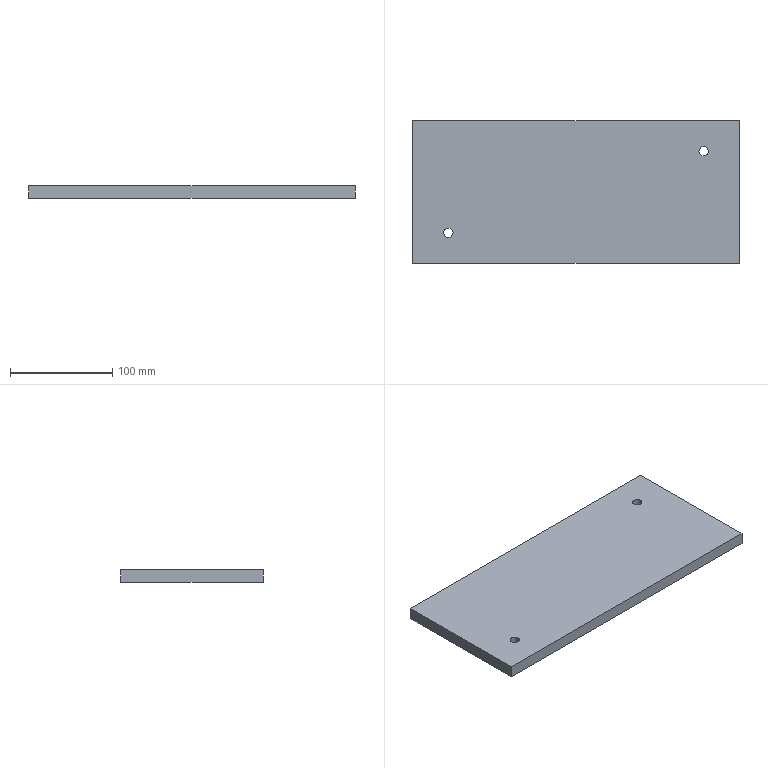Part | SolidWorks | features Extrusion 1, ICE 1 | 1 solid | 10 faces | box 320 x 140 x 12 mm | volume 536073 mm3 | plane 6 | cylinder 4 | commonest cylinder face diameters 9 x4
STEP:
#1=CARTESIAN_POINT('',(-129.5,-40.,-6.));
#2=VERTEX_POINT('',#1);
#3=CARTESIAN_POINT('',(-120.5,-40.,-6.));
#4=VERTEX_POINT('',#3);
#5=CARTESIAN_POINT('',(-125.,-40.,-6.));
#6=DIRECTION('',(0.,0.,1.));
#7=DIRECTION('',(1.,0.,0.));
#8=AXIS2_PLACEMENT_3D('',#5,#6,#7);
#9=CIRCLE('',#8,4.5);
#10=EDGE_CURVE('',#2,#4,#9,.T.);
#11=ORIENTED_EDGE('',*,*,#10,.F.);
#12=CARTESIAN_POINT('',(-129.5,-40.,6.));
#13=VERTEX_POINT('',#12);
#14=CARTESIAN_POINT('',(-129.5,-40.,-16.));
#15=DIRECTION('',(0.,0.,1.));
#16=VECTOR('',#15,1000.);
#17=LINE('',#14,#16);
#18=EDGE_CURVE('',#2,#13,#17,.T.);
#19=ORIENTED_EDGE('',*,*,#18,.T.);
#20=CARTESIAN_POINT('',(-120.5,-40.,6.));
#21=VERTEX_POINT('',#20);
#22=CARTESIAN_POINT('',(-125.,-40.,6.));
#23=DIRECTION('',(0.,0.,1.));
#24=DIRECTION('',(1.,0.,0.));
#25=AXIS2_PLACEMENT_3D('',#22,#23,#24);
#26=CIRCLE('',#25,4.5);
#27=EDGE_CURVE('',#13,#21,#26,.T.);
#28=ORIENTED_EDGE('',*,*,#27,.T.);
#29=CARTESIAN_POINT('',(-120.5,-40.,-16.));
#30=DIRECTION('',(0.,0.,1.));
#31=VECTOR('',#30,1000.);
#32=LINE('',#29,#31);
#33=EDGE_CURVE('',#4,#21,#32,.T.);
#34=ORIENTED_EDGE('',*,*,#33,.F.);
#35=EDGE_LOOP('',(#11,#19,#28,#34));
#36=FACE_OUTER_BOUND('',#35,.T.);
#37=CARTESIAN_POINT('',(-125.,-40.,-16.));
#38=DIRECTION('',(0.,0.,1.));
#39=DIRECTION('',(1.,0.,0.));
#40=AXIS2_PLACEMENT_3D('',#37,#38,#39);
#41=CYLINDRICAL_SURFACE('',#40,4.5);
#42=ADVANCED_FACE('',(#36),#41,.F.);
#43=CARTESIAN_POINT('',(120.5,40.,-6.));
#44=VERTEX_POINT('',#43);
#45=CARTESIAN_POINT('',(129.5,40.,-6.));
#46=VERTEX_POINT('',#45);
#47=CARTESIAN_POINT('',(125.,40.,-6.));
#48=DIRECTION('',(0.,0.,1.));
#49=DIRECTION('',(1.,0.,0.));
#50=AXIS2_PLACEMENT_3D('',#47,#48,#49);
#51=CIRCLE('',#50,4.5);
#52=EDGE_CURVE('',#44,#46,#51,.T.);
#53=ORIENTED_EDGE('',*,*,#52,.F.);
#54=CARTESIAN_POINT('',(120.5,40.,6.));
#55=VERTEX_POINT('',#54);
#56=CARTESIAN_POINT('',(120.5,40.,-16.));
#57=DIRECTION('',(0.,0.,1.));
#58=VECTOR('',#57,1000.);
#59=LINE('',#56,#58);
#60=EDGE_CURVE('',#44,#55,#59,.T.);
#61=ORIENTED_EDGE('',*,*,#60,.T.);
#62=CARTESIAN_POINT('',(129.5,40.,6.));
#63=VERTEX_POINT('',#62);
#64=CARTESIAN_POINT('',(125.,40.,6.));
#65=DIRECTION('',(0.,0.,1.));
#66=DIRECTION('',(1.,0.,0.));
#67=AXIS2_PLACEMENT_3D('',#64,#65,#66);
#68=CIRCLE('',#67,4.5);
#69=EDGE_CURVE('',#55,#63,#68,.T.);
#70=ORIENTED_EDGE('',*,*,#69,.T.);
#71=CARTESIAN_POINT('',(129.5,40.,-16.));
#72=DIRECTION('',(0.,0.,1.));
#73=VECTOR('',#72,1000.);
#74=LINE('',#71,#73);
#75=EDGE_CURVE('',#46,#63,#74,.T.);
#76=ORIENTED_EDGE('',*,*,#75,.F.);
#77=EDGE_LOOP('',(#53,#61,#70,#76));
#78=FACE_OUTER_BOUND('',#77,.T.);
#79=CARTESIAN_POINT('',(125.,40.,-16.));
#80=DIRECTION('',(0.,0.,1.));
#81=DIRECTION('',(1.,0.,0.));
#82=AXIS2_PLACEMENT_3D('',#79,#80,#81);
#83=CYLINDRICAL_SURFACE('',#82,4.5);
#84=ADVANCED_FACE('',(#78),#83,.F.);
#85=CARTESIAN_POINT('',(-160.,70.,6.));
#86=VERTEX_POINT('',#85);
#87=CARTESIAN_POINT('',(-160.,-70.,6.));
#88=VERTEX_POINT('',#87);
#89=CARTESIAN_POINT('',(-160.,70.,6.));
#90=DIRECTION('',(0.,-1.,0.));
#91=VECTOR('',#90,1000.);
#92=LINE('',#89,#91);
#93=EDGE_CURVE('',#86,#88,#92,.T.);
#94=ORIENTED_EDGE('',*,*,#93,.F.);
#95=CARTESIAN_POINT('',(-160.,70.,-6.));
#96=VERTEX_POINT('',#95);
#97=CARTESIAN_POINT('',(-160.,70.,-6.));
#98=DIRECTION('',(0.,0.,1.));
#99=VECTOR('',#98,1000.);
#100=LINE('',#97,#99);
#101=EDGE_CURVE('',#96,#86,#100,.T.);
#102=ORIENTED_EDGE('',*,*,#101,.F.);
#103=CARTESIAN_POINT('',(-160.,-70.,-6.));
#104=VERTEX_POINT('',#103);
#105=CARTESIAN_POINT('',(-160.,70.,-6.));
#106=DIRECTION('',(0.,-1.,0.));
#107=VECTOR('',#106,1000.);
#108=LINE('',#105,#107);
#109=EDGE_CURVE('',#96,#104,#108,.T.);
#110=ORIENTED_EDGE('',*,*,#109,.T.);
#111=CARTESIAN_POINT('',(-160.,-70.,-6.));
#112=DIRECTION('',(0.,0.,1.));
#113=VECTOR('',#112,1000.);
#114=LINE('',#111,#113);
#115=EDGE_CURVE('',#104,#88,#114,.T.);
#116=ORIENTED_EDGE('',*,*,#115,.T.);
#117=EDGE_LOOP('',(#94,#102,#110,#116));
#118=FACE_OUTER_BOUND('',#117,.T.);
#119=CARTESIAN_POINT('',(-160.,70.,-6.));
#120=DIRECTION('',(-1.,0.,0.));
#121=DIRECTION('',(0.,0.,1.));
#122=AXIS2_PLACEMENT_3D('',#119,#120,#121);
#123=PLANE('',#122);
#124=ADVANCED_FACE('',(#118),#123,.T.);
#125=CARTESIAN_POINT('',(160.,70.,6.));
#126=VERTEX_POINT('',#125);
#127=CARTESIAN_POINT('',(160.,70.,6.));
#128=DIRECTION('',(-1.,0.,0.));
#129=VECTOR('',#128,1000.);
#130=LINE('',#127,#129);
#131=EDGE_CURVE('',#126,#86,#130,.T.);
#132=ORIENTED_EDGE('',*,*,#131,.F.);
#133=CARTESIAN_POINT('',(160.,70.,-6.));
#134=VERTEX_POINT('',#133);
#135=CARTESIAN_POINT('',(160.,70.,-6.));
#136=DIRECTION('',(0.,0.,1.));
#137=VECTOR('',#136,1000.);
#138=LINE('',#135,#137);
#139=EDGE_CURVE('',#134,#126,#138,.T.);
#140=ORIENTED_EDGE('',*,*,#139,.F.);
#141=CARTESIAN_POINT('',(160.,70.,-6.));
#142=DIRECTION('',(-1.,0.,0.));
#143=VECTOR('',#142,1000.);
#144=LINE('',#141,#143);
#145=EDGE_CURVE('',#134,#96,#144,.T.);
#146=ORIENTED_EDGE('',*,*,#145,.T.);
#147=ORIENTED_EDGE('',*,*,#101,.T.);
#148=EDGE_LOOP('',(#132,#140,#146,#147));
#149=FACE_OUTER_BOUND('',#148,.T.);
#150=CARTESIAN_POINT('',(160.,70.,-6.));
#151=DIRECTION('',(0.,1.,0.));
#152=DIRECTION('',(0.,0.,1.));
#153=AXIS2_PLACEMENT_3D('',#150,#151,#152);
#154=PLANE('',#153);
#155=ADVANCED_FACE('',(#149),#154,.T.);
#156=CARTESIAN_POINT('',(160.,-70.,6.));
#157=VERTEX_POINT('',#156);
#158=CARTESIAN_POINT('',(160.,-70.,6.));
#159=DIRECTION('',(0.,1.,0.));
#160=VECTOR('',#159,1000.);
#161=LINE('',#158,#160);
#162=EDGE_CURVE('',#157,#126,#161,.T.);
#163=ORIENTED_EDGE('',*,*,#162,.F.);
#164=CARTESIAN_POINT('',(160.,-70.,-6.));
#165=VERTEX_POINT('',#164);
#166=CARTESIAN_POINT('',(160.,-70.,-6.));
#167=DIRECTION('',(0.,0.,1.));
#168=VECTOR('',#167,1000.);
#169=LINE('',#166,#168);
#170=EDGE_CURVE('',#165,#157,#169,.T.);
#171=ORIENTED_EDGE('',*,*,#170,.F.);
#172=CARTESIAN_POINT('',(160.,-70.,-6.));
#173=DIRECTION('',(0.,1.,0.));
#174=VECTOR('',#173,1000.);
#175=LINE('',#172,#174);
#176=EDGE_CURVE('',#165,#134,#175,.T.);
#177=ORIENTED_EDGE('',*,*,#176,.T.);
#178=ORIENTED_EDGE('',*,*,#139,.T.);
#179=EDGE_LOOP('',(#163,#171,#177,#178));
#180=FACE_OUTER_BOUND('',#179,.T.);
#181=CARTESIAN_POINT('',(160.,-70.,-6.));
#182=DIRECTION('',(1.,0.,0.));
#183=DIRECTION('',(0.,0.,-1.));
#184=AXIS2_PLACEMENT_3D('',#181,#182,#183);
#185=PLANE('',#184);
#186=ADVANCED_FACE('',(#180),#185,.T.);
#187=CARTESIAN_POINT('',(-160.,-70.,6.));
#188=DIRECTION('',(1.,0.,0.));
#189=VECTOR('',#188,1000.);
#190=LINE('',#187,#189);
#191=EDGE_CURVE('',#88,#157,#190,.T.);
#192=ORIENTED_EDGE('',*,*,#191,.F.);
#193=ORIENTED_EDGE('',*,*,#115,.F.);
#194=CARTESIAN_POINT('',(-160.,-70.,-6.));
#195=DIRECTION('',(1.,0.,0.));
#196=VECTOR('',#195,1000.);
#197=LINE('',#194,#196);
#198=EDGE_CURVE('',#104,#165,#197,.T.);
#199=ORIENTED_EDGE('',*,*,#198,.T.);
#200=ORIENTED_EDGE('',*,*,#170,.T.);
#201=EDGE_LOOP('',(#192,#193,#199,#200));
#202=FACE_OUTER_BOUND('',#201,.T.);
#203=CARTESIAN_POINT('',(-160.,-70.,-6.));
#204=DIRECTION('',(0.,-1.,0.));
#205=DIRECTION('',(0.,0.,-1.));
#206=AXIS2_PLACEMENT_3D('',#203,#204,#205);
#207=PLANE('',#206);
#208=ADVANCED_FACE('',(#202),#207,.T.);
#209=CARTESIAN_POINT('',(-125.,-40.,-6.));
#210=DIRECTION('',(0.,0.,1.));
#211=DIRECTION('',(1.,0.,0.));
#212=AXIS2_PLACEMENT_3D('',#209,#210,#211);
#213=CIRCLE('',#212,4.5);
#214=EDGE_CURVE('',#4,#2,#213,.T.);
#215=ORIENTED_EDGE('',*,*,#214,.T.);
#216=ORIENTED_EDGE('',*,*,#10,.T.);
#217=EDGE_LOOP('',(#215,#216));
#218=FACE_BOUND('',#217,.T.);
#219=CARTESIAN_POINT('',(125.,40.,-6.));
#220=DIRECTION('',(0.,0.,1.));
#221=DIRECTION('',(1.,0.,0.));
#222=AXIS2_PLACEMENT_3D('',#219,#220,#221);
#223=CIRCLE('',#222,4.5);
#224=EDGE_CURVE('',#46,#44,#223,.T.);
#225=ORIENTED_EDGE('',*,*,#224,.T.);
#226=ORIENTED_EDGE('',*,*,#52,.T.);
#227=EDGE_LOOP('',(#225,#226));
#228=FACE_BOUND('',#227,.T.);
#229=ORIENTED_EDGE('',*,*,#109,.F.);
#230=ORIENTED_EDGE('',*,*,#145,.F.);
#231=ORIENTED_EDGE('',*,*,#176,.F.);
#232=ORIENTED_EDGE('',*,*,#198,.F.);
#233=EDGE_LOOP('',(#229,#230,#231,#232));
#234=FACE_OUTER_BOUND('',#233,.T.);
#235=CARTESIAN_POINT('',(0.,0.,-6.));
#236=DIRECTION('',(0.,0.,1.));
#237=DIRECTION('',(1.,0.,0.));
#238=AXIS2_PLACEMENT_3D('',#235,#236,#237);
#239=PLANE('',#238);
#240=ADVANCED_FACE('',(#218,#228,#234),#239,.F.);
#241=CARTESIAN_POINT('',(-125.,-40.,6.));
#242=DIRECTION('',(0.,0.,1.));
#243=DIRECTION('',(1.,0.,0.));
#244=AXIS2_PLACEMENT_3D('',#241,#242,#243);
#245=CIRCLE('',#244,4.5);
#246=EDGE_CURVE('',#21,#13,#245,.T.);
#247=ORIENTED_EDGE('',*,*,#246,.F.);
#248=ORIENTED_EDGE('',*,*,#27,.F.);
#249=EDGE_LOOP('',(#247,#248));
#250=FACE_BOUND('',#249,.T.);
#251=CARTESIAN_POINT('',(125.,40.,6.));
#252=DIRECTION('',(0.,0.,1.));
#253=DIRECTION('',(1.,0.,0.));
#254=AXIS2_PLACEMENT_3D('',#251,#252,#253);
#255=CIRCLE('',#254,4.5);
#256=EDGE_CURVE('',#63,#55,#255,.T.);
#257=ORIENTED_EDGE('',*,*,#256,.F.);
#258=ORIENTED_EDGE('',*,*,#69,.F.);
#259=EDGE_LOOP('',(#257,#258));
#260=FACE_BOUND('',#259,.T.);
#261=ORIENTED_EDGE('',*,*,#93,.T.);
#262=ORIENTED_EDGE('',*,*,#191,.T.);
#263=ORIENTED_EDGE('',*,*,#162,.T.);
#264=ORIENTED_EDGE('',*,*,#131,.T.);
#265=EDGE_LOOP('',(#261,#262,#263,#264));
#266=FACE_OUTER_BOUND('',#265,.T.);
#267=CARTESIAN_POINT('',(0.,0.,6.));
#268=DIRECTION('',(0.,0.,1.));
#269=DIRECTION('',(1.,0.,0.));
#270=AXIS2_PLACEMENT_3D('',#267,#268,#269);
#271=PLANE('',#270);
#272=ADVANCED_FACE('',(#250,#260,#266),#271,.T.);
#273=ORIENTED_EDGE('',*,*,#60,.F.);
#274=ORIENTED_EDGE('',*,*,#224,.F.);
#275=ORIENTED_EDGE('',*,*,#75,.T.);
#276=ORIENTED_EDGE('',*,*,#256,.T.);
#277=EDGE_LOOP('',(#273,#274,#275,#276));
#278=FACE_OUTER_BOUND('',#277,.T.);
#279=CARTESIAN_POINT('',(125.,40.,-16.));
#280=DIRECTION('',(0.,0.,1.));
#281=DIRECTION('',(1.,0.,0.));
#282=AXIS2_PLACEMENT_3D('',#279,#280,#281);
#283=CYLINDRICAL_SURFACE('',#282,4.5);
#284=ADVANCED_FACE('',(#278),#283,.F.);
#285=ORIENTED_EDGE('',*,*,#18,.F.);
#286=ORIENTED_EDGE('',*,*,#214,.F.);
#287=ORIENTED_EDGE('',*,*,#33,.T.);
#288=ORIENTED_EDGE('',*,*,#246,.T.);
#289=EDGE_LOOP('',(#285,#286,#287,#288));
#290=FACE_OUTER_BOUND('',#289,.T.);
#291=CARTESIAN_POINT('',(-125.,-40.,-16.));
#292=DIRECTION('',(0.,0.,1.));
#293=DIRECTION('',(1.,0.,0.));
#294=AXIS2_PLACEMENT_3D('',#291,#292,#293);
#295=CYLINDRICAL_SURFACE('',#294,4.5);
#296=ADVANCED_FACE('',(#290),#295,.F.);
#297=CLOSED_SHELL('',(#42,#84,#124,#155,#186,#208,#240,#272,#284,#296));
#298=MANIFOLD_SOLID_BREP('',#297);
#299=CARTESIAN_POINT('',(0.,0.,0.));
#300=DIRECTION('',(0.,0.,1.));
#301=DIRECTION('',(1.,0.,0.));
#302=AXIS2_PLACEMENT_3D('',#299,#300,#301);
#303=(LENGTH_UNIT()NAMED_UNIT(*)SI_UNIT(.MILLI.,.METRE.));
#304=UNCERTAINTY_MEASURE_WITH_UNIT(LENGTH_MEASURE(0.00001),#303,'','');
#305=(NAMED_UNIT(*)PLANE_ANGLE_UNIT()SI_UNIT($,.RADIAN.));
#306=(NAMED_UNIT(*)SI_UNIT($,.STERADIAN.)SOLID_ANGLE_UNIT());
#307=(GEOMETRIC_REPRESENTATION_CONTEXT(3)GLOBAL_UNCERTAINTY_ASSIGNED_CONTEXT((#304))GLOBAL_UNIT_ASSIGNED_CONTEXT((#303,#305,#306))REPRESENTATION_CONTEXT('',''));
#308=ADVANCED_BREP_SHAPE_REPRESENTATION('',(#298,#302),#307);